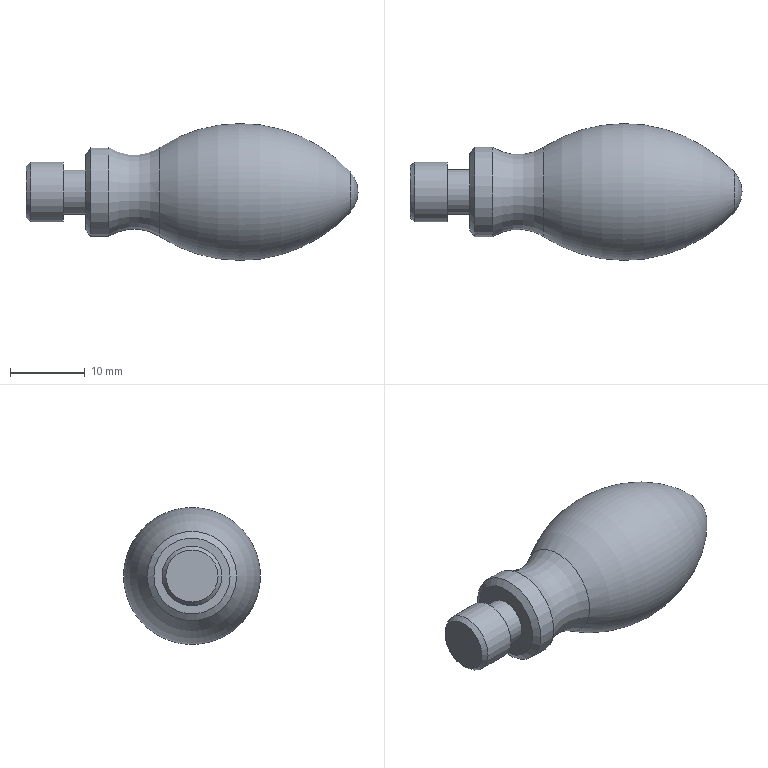Part | NX | features CHAMFER 2, DATUM_CSYS 2, SKETCH 1, SWP104 1 | 1 solid | 11 faces | box 44.482 x 18.329 x 18.329 mm | volume 6113 mm3 | plane 3 | cylinder 3 | torus 2 | cone 2 | sphere 1 | commonest cylinder face diameters 6 x1 8 x1 12 x1
STEP:
#1=CARTESIAN_POINT('',(43.426,-2.709,0.));
#2=VERTEX_POINT('',#1);
#3=CARTESIAN_POINT('',(43.426,0.,0.));
#4=DIRECTION('',(-1.,0.,0.));
#5=DIRECTION('',(0.,-1.,0.));
#6=AXIS2_PLACEMENT_3D('',#3,#4,#5);
#7=CIRCLE('',#6,2.709);
#8=EDGE_CURVE('',#2,#2,#7,.T.);
#9=ORIENTED_EDGE('',*,*,#8,.T.);
#10=EDGE_LOOP('',(#9));
#11=FACE_BOUND('',#10,.T.);
#12=CARTESIAN_POINT('',(17.914,-6.,0.));
#13=VERTEX_POINT('',#12);
#14=CARTESIAN_POINT('',(17.914,0.,0.));
#15=DIRECTION('',(-1.,0.,0.));
#16=DIRECTION('',(0.,-1.,0.));
#17=AXIS2_PLACEMENT_3D('',#14,#15,#16);
#18=CIRCLE('',#17,6.);
#19=EDGE_CURVE('',#13,#13,#18,.T.);
#20=ORIENTED_EDGE('',*,*,#19,.F.);
#21=EDGE_LOOP('',(#20));
#22=FACE_BOUND('',#21,.T.);
#23=CARTESIAN_POINT('',(28.71,0.,0.));
#24=DIRECTION('',(-1.,0.,0.));
#25=DIRECTION('',(0.,-1.,0.));
#26=AXIS2_PLACEMENT_3D('',#23,#24,#25);
#27=DEGENERATE_TOROIDAL_SURFACE('',#26,10.836,20.,.F.);
#28=ADVANCED_FACE('',(#11,#22),#27,.F.);
#29=ORIENTED_EDGE('',*,*,#8,.F.);
#30=EDGE_LOOP('',(#29));
#31=FACE_BOUND('',#30,.T.);
#32=CARTESIAN_POINT('',(40.482,0.,0.));
#33=DIRECTION('',(-1.,0.,0.));
#34=DIRECTION('',(0.,1.,0.));
#35=AXIS2_PLACEMENT_3D('',#32,#33,#34);
#36=SPHERICAL_SURFACE('',#35,4.);
#37=ADVANCED_FACE('',(#31),#36,.T.);
#38=CARTESIAN_POINT('',(0.,-3.5,0.));
#39=VERTEX_POINT('',#38);
#40=CARTESIAN_POINT('',(0.,0.,0.));
#41=DIRECTION('',(-1.,0.,0.));
#42=DIRECTION('',(0.,-1.,0.));
#43=AXIS2_PLACEMENT_3D('',#40,#41,#42);
#44=CIRCLE('',#43,3.5);
#45=EDGE_CURVE('',#39,#39,#44,.T.);
#46=ORIENTED_EDGE('',*,*,#45,.T.);
#47=EDGE_LOOP('',(#46));
#48=FACE_BOUND('',#47,.T.);
#49=CARTESIAN_POINT('',(0.,0.,0.));
#50=DIRECTION('',(-1.,0.,0.));
#51=DIRECTION('',(0.,-1.,0.));
#52=AXIS2_PLACEMENT_3D('',#49,#50,#51);
#53=PLANE('',#52);
#54=ADVANCED_FACE('',(#48),#53,.T.);
#55=CARTESIAN_POINT('',(0.65,-4.,0.));
#56=VERTEX_POINT('',#55);
#57=CARTESIAN_POINT('',(0.65,0.,0.));
#58=DIRECTION('',(-1.,0.,0.));
#59=DIRECTION('',(0.,-1.,0.));
#60=AXIS2_PLACEMENT_3D('',#57,#58,#59);
#61=CIRCLE('',#60,4.);
#62=EDGE_CURVE('',#56,#56,#61,.F.);
#63=ORIENTED_EDGE('',*,*,#62,.T.);
#64=EDGE_LOOP('',(#63));
#65=FACE_BOUND('',#64,.T.);
#66=CARTESIAN_POINT('',(5.,-4.,0.));
#67=VERTEX_POINT('',#66);
#68=CARTESIAN_POINT('',(5.,0.,0.));
#69=DIRECTION('',(-1.,0.,0.));
#70=DIRECTION('',(0.,-1.,0.));
#71=AXIS2_PLACEMENT_3D('',#68,#69,#70);
#72=CIRCLE('',#71,4.);
#73=EDGE_CURVE('',#67,#67,#72,.T.);
#74=ORIENTED_EDGE('',*,*,#73,.T.);
#75=EDGE_LOOP('',(#74));
#76=FACE_BOUND('',#75,.T.);
#77=CARTESIAN_POINT('',(44.482,0.,0.));
#78=DIRECTION('',(-1.,0.,0.));
#79=DIRECTION('',(0.,-1.,0.));
#80=AXIS2_PLACEMENT_3D('',#77,#78,#79);
#81=CYLINDRICAL_SURFACE('',#80,4.);
#82=ADVANCED_FACE('',(#65,#76),#81,.T.);
#83=CARTESIAN_POINT('',(5.,-3.,0.));
#84=VERTEX_POINT('',#83);
#85=CARTESIAN_POINT('',(5.,0.,0.));
#86=DIRECTION('',(-1.,0.,0.));
#87=DIRECTION('',(0.,-1.,0.));
#88=AXIS2_PLACEMENT_3D('',#85,#86,#87);
#89=CIRCLE('',#88,3.);
#90=EDGE_CURVE('',#84,#84,#89,.T.);
#91=ORIENTED_EDGE('',*,*,#90,.T.);
#92=EDGE_LOOP('',(#91));
#93=FACE_BOUND('',#92,.T.);
#94=ORIENTED_EDGE('',*,*,#73,.F.);
#95=EDGE_LOOP('',(#94));
#96=FACE_BOUND('',#95,.T.);
#97=CARTESIAN_POINT('',(5.,4.,0.));
#98=DIRECTION('',(1.,0.,0.));
#99=DIRECTION('',(0.,1.,0.));
#100=AXIS2_PLACEMENT_3D('',#97,#98,#99);
#101=PLANE('',#100);
#102=ADVANCED_FACE('',(#93,#96),#101,.T.);
#103=CARTESIAN_POINT('',(8.,-3.,0.));
#104=VERTEX_POINT('',#103);
#105=CARTESIAN_POINT('',(8.,0.,0.));
#106=DIRECTION('',(-1.,0.,0.));
#107=DIRECTION('',(0.,-1.,0.));
#108=AXIS2_PLACEMENT_3D('',#105,#106,#107);
#109=CIRCLE('',#108,3.);
#110=EDGE_CURVE('',#104,#104,#109,.T.);
#111=ORIENTED_EDGE('',*,*,#110,.T.);
#112=EDGE_LOOP('',(#111));
#113=FACE_BOUND('',#112,.T.);
#114=ORIENTED_EDGE('',*,*,#90,.F.);
#115=EDGE_LOOP('',(#114));
#116=FACE_BOUND('',#115,.T.);
#117=CARTESIAN_POINT('',(44.482,0.,0.));
#118=DIRECTION('',(-1.,0.,0.));
#119=DIRECTION('',(0.,-1.,0.));
#120=AXIS2_PLACEMENT_3D('',#117,#118,#119);
#121=CYLINDRICAL_SURFACE('',#120,3.);
#122=ADVANCED_FACE('',(#113,#116),#121,.T.);
#123=CARTESIAN_POINT('',(8.,-5.1,0.));
#124=VERTEX_POINT('',#123);
#125=CARTESIAN_POINT('',(8.,0.,0.));
#126=DIRECTION('',(-1.,0.,0.));
#127=DIRECTION('',(0.,-1.,0.));
#128=AXIS2_PLACEMENT_3D('',#125,#126,#127);
#129=CIRCLE('',#128,5.1);
#130=EDGE_CURVE('',#124,#124,#129,.T.);
#131=ORIENTED_EDGE('',*,*,#130,.T.);
#132=EDGE_LOOP('',(#131));
#133=FACE_BOUND('',#132,.T.);
#134=ORIENTED_EDGE('',*,*,#110,.F.);
#135=EDGE_LOOP('',(#134));
#136=FACE_BOUND('',#135,.T.);
#137=CARTESIAN_POINT('',(8.,3.,0.));
#138=DIRECTION('',(-1.,0.,0.));
#139=DIRECTION('',(0.,-1.,0.));
#140=AXIS2_PLACEMENT_3D('',#137,#138,#139);
#141=PLANE('',#140);
#142=ADVANCED_FACE('',(#133,#136),#141,.T.);
#143=CARTESIAN_POINT('',(8.65,-6.,0.));
#144=VERTEX_POINT('',#143);
#145=CARTESIAN_POINT('',(8.65,0.,0.));
#146=DIRECTION('',(-1.,0.,0.));
#147=DIRECTION('',(0.,-1.,0.));
#148=AXIS2_PLACEMENT_3D('',#145,#146,#147);
#149=CIRCLE('',#148,6.);
#150=EDGE_CURVE('',#144,#144,#149,.F.);
#151=ORIENTED_EDGE('',*,*,#150,.T.);
#152=EDGE_LOOP('',(#151));
#153=FACE_BOUND('',#152,.T.);
#154=CARTESIAN_POINT('',(11.09,-6.,0.));
#155=VERTEX_POINT('',#154);
#156=CARTESIAN_POINT('',(11.09,0.,0.));
#157=DIRECTION('',(-1.,0.,0.));
#158=DIRECTION('',(0.,-1.,0.));
#159=AXIS2_PLACEMENT_3D('',#156,#157,#158);
#160=CIRCLE('',#159,6.);
#161=EDGE_CURVE('',#155,#155,#160,.T.);
#162=ORIENTED_EDGE('',*,*,#161,.T.);
#163=EDGE_LOOP('',(#162));
#164=FACE_BOUND('',#163,.T.);
#165=CARTESIAN_POINT('',(44.482,0.,0.));
#166=DIRECTION('',(-1.,0.,0.));
#167=DIRECTION('',(0.,-1.,0.));
#168=AXIS2_PLACEMENT_3D('',#165,#166,#167);
#169=CYLINDRICAL_SURFACE('',#168,6.);
#170=ADVANCED_FACE('',(#153,#164),#169,.T.);
#171=ORIENTED_EDGE('',*,*,#19,.T.);
#172=EDGE_LOOP('',(#171));
#173=FACE_BOUND('',#172,.T.);
#174=ORIENTED_EDGE('',*,*,#161,.F.);
#175=EDGE_LOOP('',(#174));
#176=FACE_BOUND('',#175,.T.);
#177=CARTESIAN_POINT('',(14.502,0.,0.));
#178=DIRECTION('',(-1.,0.,0.));
#179=DIRECTION('',(0.,-1.,0.));
#180=AXIS2_PLACEMENT_3D('',#177,#178,#179);
#181=TOROIDAL_SURFACE('',#180,11.32,6.32);
#182=ADVANCED_FACE('',(#173,#176),#181,.F.);
#183=ORIENTED_EDGE('',*,*,#150,.F.);
#184=EDGE_LOOP('',(#183));
#185=FACE_BOUND('',#184,.T.);
#186=ORIENTED_EDGE('',*,*,#130,.F.);
#187=EDGE_LOOP('',(#186));
#188=FACE_BOUND('',#187,.T.);
#189=CARTESIAN_POINT('',(8.,0.,0.));
#190=DIRECTION('',(1.,0.,0.));
#191=DIRECTION('',(0.,1.,0.));
#192=AXIS2_PLACEMENT_3D('',#189,#190,#191);
#193=CONICAL_SURFACE('',#192,5.1,0.9453);
#194=ADVANCED_FACE('',(#185,#188),#193,.T.);
#195=ORIENTED_EDGE('',*,*,#62,.F.);
#196=EDGE_LOOP('',(#195));
#197=FACE_BOUND('',#196,.T.);
#198=ORIENTED_EDGE('',*,*,#45,.F.);
#199=EDGE_LOOP('',(#198));
#200=FACE_BOUND('',#199,.T.);
#201=CARTESIAN_POINT('',(0.,0.,0.));
#202=DIRECTION('',(1.,0.,0.));
#203=DIRECTION('',(0.,1.,0.));
#204=AXIS2_PLACEMENT_3D('',#201,#202,#203);
#205=CONICAL_SURFACE('',#204,3.5,0.6557);
#206=ADVANCED_FACE('',(#197,#200),#205,.T.);
#207=CLOSED_SHELL('',(#28,#37,#54,#82,#102,#122,#142,#170,#182,#194,#206));
#208=MANIFOLD_SOLID_BREP('',#207);
#209=(LENGTH_UNIT()NAMED_UNIT(*)SI_UNIT(.MILLI.,.METRE.));
#210=UNCERTAINTY_MEASURE_WITH_UNIT(LENGTH_MEASURE(0.00001),#209,'','');
#211=(NAMED_UNIT(*)PLANE_ANGLE_UNIT()SI_UNIT($,.RADIAN.));
#212=(NAMED_UNIT(*)SI_UNIT($,.STERADIAN.)SOLID_ANGLE_UNIT());
#213=(GEOMETRIC_REPRESENTATION_CONTEXT(3)GLOBAL_UNCERTAINTY_ASSIGNED_CONTEXT((#210))GLOBAL_UNIT_ASSIGNED_CONTEXT((#209,#211,#212))REPRESENTATION_CONTEXT('',''));
#214=ADVANCED_BREP_SHAPE_REPRESENTATION('',(#208),#213);